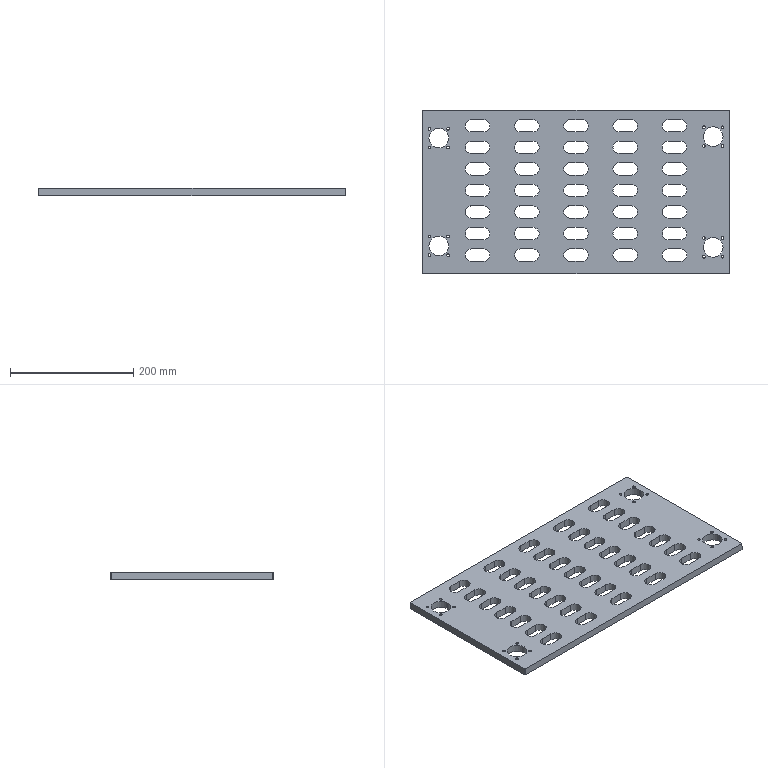Part | STEP file | X77-09001 | 1 solid | 225 faces | box 500 x 265 x 12 mm | volume 1248765 mm3 | cylinder 145 | plane 80 | commonest cylinder face diameters 20 x105 4.2 x32 32 x8